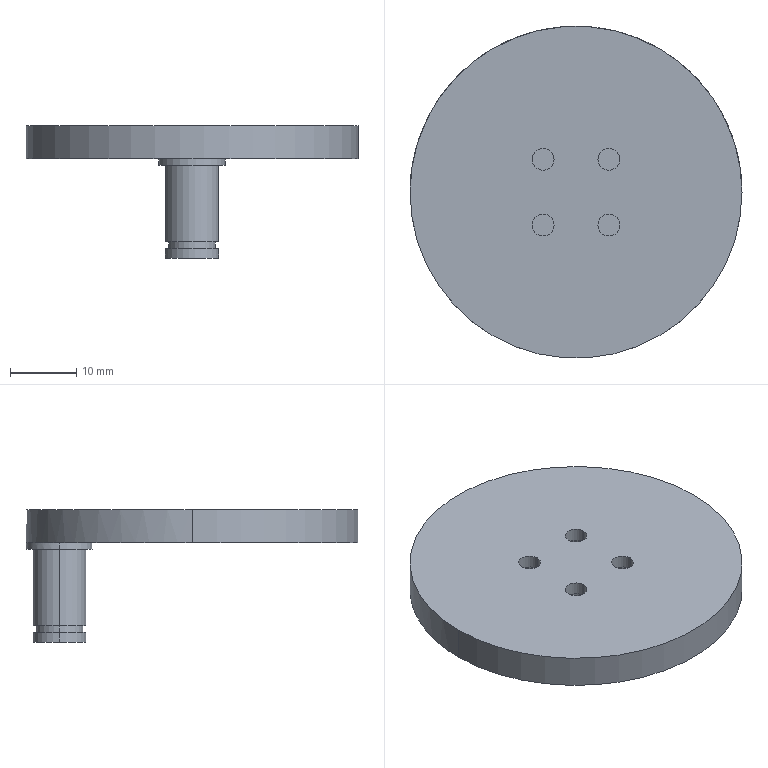Part | SolidWorks | features MirrorStock 1 | 1 solid | 36 faces | box 50 x 50 x 20 mm | volume 10180 mm3 | cylinder 26 | plane 10 | commonest cylinder face diameters 3.3 x8 6 x8 8 x4 7 x2 10 x2 50 x2
STEP:
#1=CARTESIAN_POINT('',(-4.,20.,-20.));
#2=VERTEX_POINT('',#1);
#3=CARTESIAN_POINT('',(4.,20.,-20.));
#4=VERTEX_POINT('',#3);
#5=CARTESIAN_POINT('',(0.,20.,-20.));
#6=DIRECTION('',(0.,0.,1.));
#7=DIRECTION('',(1.,0.,0.));
#8=AXIS2_PLACEMENT_3D('',#5,#6,#7);
#9=CIRCLE('',#8,4.);
#10=EDGE_CURVE('',#2,#4,#9,.T.);
#11=ORIENTED_EDGE('',*,*,#10,.T.);
#12=CARTESIAN_POINT('',(4.,20.,-18.5));
#13=VERTEX_POINT('',#12);
#14=CARTESIAN_POINT('',(4.,20.,-20.));
#15=DIRECTION('',(0.,0.,1.));
#16=VECTOR('',#15,1000.);
#17=LINE('',#14,#16);
#18=EDGE_CURVE('',#4,#13,#17,.T.);
#19=ORIENTED_EDGE('',*,*,#18,.T.);
#20=CARTESIAN_POINT('',(-4.,20.,-18.5));
#21=VERTEX_POINT('',#20);
#22=CARTESIAN_POINT('',(0.,20.,-18.5));
#23=DIRECTION('',(0.,0.,1.));
#24=DIRECTION('',(1.,0.,0.));
#25=AXIS2_PLACEMENT_3D('',#22,#23,#24);
#26=CIRCLE('',#25,4.);
#27=EDGE_CURVE('',#21,#13,#26,.T.);
#28=ORIENTED_EDGE('',*,*,#27,.F.);
#29=CARTESIAN_POINT('',(-4.,20.,-20.));
#30=DIRECTION('',(0.,0.,1.));
#31=VECTOR('',#30,1000.);
#32=LINE('',#29,#31);
#33=EDGE_CURVE('',#2,#21,#32,.T.);
#34=ORIENTED_EDGE('',*,*,#33,.F.);
#35=EDGE_LOOP('',(#11,#19,#28,#34));
#36=FACE_OUTER_BOUND('',#35,.T.);
#37=CARTESIAN_POINT('',(0.,20.,-20.));
#38=DIRECTION('',(0.,0.,1.));
#39=DIRECTION('',(-1.,0.,0.));
#40=AXIS2_PLACEMENT_3D('',#37,#38,#39);
#41=CYLINDRICAL_SURFACE('',#40,4.);
#42=ADVANCED_FACE('',(#36),#41,.T.);
#43=CARTESIAN_POINT('',(-3.5,20.,-17.5));
#44=VERTEX_POINT('',#43);
#45=CARTESIAN_POINT('',(3.5,20.,-17.5));
#46=VERTEX_POINT('',#45);
#47=CARTESIAN_POINT('',(0.,20.,-17.5));
#48=DIRECTION('',(0.,0.,1.));
#49=DIRECTION('',(1.,0.,0.));
#50=AXIS2_PLACEMENT_3D('',#47,#48,#49);
#51=CIRCLE('',#50,3.5);
#52=EDGE_CURVE('',#44,#46,#51,.T.);
#53=ORIENTED_EDGE('',*,*,#52,.F.);
#54=CARTESIAN_POINT('',(-3.5,20.,-18.5));
#55=VERTEX_POINT('',#54);
#56=CARTESIAN_POINT('',(-3.5,20.,-17.5));
#57=DIRECTION('',(0.,0.,-1.));
#58=VECTOR('',#57,1000.);
#59=LINE('',#56,#58);
#60=EDGE_CURVE('',#44,#55,#59,.T.);
#61=ORIENTED_EDGE('',*,*,#60,.T.);
#62=CARTESIAN_POINT('',(3.5,20.,-18.5));
#63=VERTEX_POINT('',#62);
#64=CARTESIAN_POINT('',(0.,20.,-18.5));
#65=DIRECTION('',(0.,0.,1.));
#66=DIRECTION('',(1.,0.,0.));
#67=AXIS2_PLACEMENT_3D('',#64,#65,#66);
#68=CIRCLE('',#67,3.5);
#69=EDGE_CURVE('',#55,#63,#68,.T.);
#70=ORIENTED_EDGE('',*,*,#69,.T.);
#71=CARTESIAN_POINT('',(3.5,20.,-17.5));
#72=DIRECTION('',(0.,0.,-1.));
#73=VECTOR('',#72,1000.);
#74=LINE('',#71,#73);
#75=EDGE_CURVE('',#46,#63,#74,.T.);
#76=ORIENTED_EDGE('',*,*,#75,.F.);
#77=EDGE_LOOP('',(#53,#61,#70,#76));
#78=FACE_OUTER_BOUND('',#77,.T.);
#79=CARTESIAN_POINT('',(0.,20.,-17.5));
#80=DIRECTION('',(0.,0.,-1.));
#81=DIRECTION('',(1.,0.,0.));
#82=AXIS2_PLACEMENT_3D('',#79,#80,#81);
#83=CYLINDRICAL_SURFACE('',#82,3.5);
#84=ADVANCED_FACE('',(#78),#83,.T.);
#85=CARTESIAN_POINT('',(-5.,20.,-6.));
#86=VERTEX_POINT('',#85);
#87=CARTESIAN_POINT('',(5.,20.,-6.));
#88=VERTEX_POINT('',#87);
#89=CARTESIAN_POINT('',(0.,20.,-6.));
#90=DIRECTION('',(0.,0.,1.));
#91=DIRECTION('',(1.,0.,0.));
#92=AXIS2_PLACEMENT_3D('',#89,#90,#91);
#93=CIRCLE('',#92,5.);
#94=EDGE_CURVE('',#86,#88,#93,.T.);
#95=ORIENTED_EDGE('',*,*,#94,.T.);
#96=CARTESIAN_POINT('',(5.,20.,-5.));
#97=VERTEX_POINT('',#96);
#98=CARTESIAN_POINT('',(5.,20.,-6.));
#99=DIRECTION('',(0.,0.,1.));
#100=VECTOR('',#99,1000.);
#101=LINE('',#98,#100);
#102=EDGE_CURVE('',#88,#97,#101,.T.);
#103=ORIENTED_EDGE('',*,*,#102,.T.);
#104=CARTESIAN_POINT('',(-5.,20.,-5.));
#105=VERTEX_POINT('',#104);
#106=CARTESIAN_POINT('',(0.,20.,-5.));
#107=DIRECTION('',(0.,0.,1.));
#108=DIRECTION('',(1.,0.,0.));
#109=AXIS2_PLACEMENT_3D('',#106,#107,#108);
#110=CIRCLE('',#109,5.);
#111=EDGE_CURVE('',#105,#97,#110,.T.);
#112=ORIENTED_EDGE('',*,*,#111,.F.);
#113=CARTESIAN_POINT('',(-5.,20.,-6.));
#114=DIRECTION('',(0.,0.,1.));
#115=VECTOR('',#114,1000.);
#116=LINE('',#113,#115);
#117=EDGE_CURVE('',#86,#105,#116,.T.);
#118=ORIENTED_EDGE('',*,*,#117,.F.);
#119=EDGE_LOOP('',(#95,#103,#112,#118));
#120=FACE_OUTER_BOUND('',#119,.T.);
#121=CARTESIAN_POINT('',(0.,20.,-6.));
#122=DIRECTION('',(0.,0.,1.));
#123=DIRECTION('',(-1.,0.,0.));
#124=AXIS2_PLACEMENT_3D('',#121,#122,#123);
#125=CYLINDRICAL_SURFACE('',#124,5.);
#126=ADVANCED_FACE('',(#120),#125,.T.);
#127=CARTESIAN_POINT('',(-7.95,4.95,-2.));
#128=VERTEX_POINT('',#127);
#129=CARTESIAN_POINT('',(-1.95,4.95,-2.));
#130=VERTEX_POINT('',#129);
#131=CARTESIAN_POINT('',(-4.95,4.95,-2.));
#132=DIRECTION('',(0.,0.,-1.));
#133=DIRECTION('',(-1.,0.,0.));
#134=AXIS2_PLACEMENT_3D('',#131,#132,#133);
#135=CIRCLE('',#134,3.);
#136=EDGE_CURVE('',#128,#130,#135,.T.);
#137=ORIENTED_EDGE('',*,*,#136,.F.);
#138=CARTESIAN_POINT('',(-7.95,4.95,-5.));
#139=VERTEX_POINT('',#138);
#140=CARTESIAN_POINT('',(-7.95,4.95,-2.));
#141=DIRECTION('',(0.,0.,-1.));
#142=VECTOR('',#141,1000.);
#143=LINE('',#140,#142);
#144=EDGE_CURVE('',#128,#139,#143,.T.);
#145=ORIENTED_EDGE('',*,*,#144,.T.);
#146=CARTESIAN_POINT('',(-1.95,4.95,-5.));
#147=VERTEX_POINT('',#146);
#148=CARTESIAN_POINT('',(-4.95,4.95,-5.));
#149=DIRECTION('',(0.,0.,-1.));
#150=DIRECTION('',(-1.,0.,0.));
#151=AXIS2_PLACEMENT_3D('',#148,#149,#150);
#152=CIRCLE('',#151,3.);
#153=EDGE_CURVE('',#139,#147,#152,.T.);
#154=ORIENTED_EDGE('',*,*,#153,.T.);
#155=CARTESIAN_POINT('',(-1.95,4.95,-2.));
#156=DIRECTION('',(0.,0.,-1.));
#157=VECTOR('',#156,1000.);
#158=LINE('',#155,#157);
#159=EDGE_CURVE('',#130,#147,#158,.T.);
#160=ORIENTED_EDGE('',*,*,#159,.F.);
#161=EDGE_LOOP('',(#137,#145,#154,#160));
#162=FACE_OUTER_BOUND('',#161,.T.);
#163=CARTESIAN_POINT('',(-4.95,4.95,-2.));
#164=DIRECTION('',(0.,0.,-1.));
#165=DIRECTION('',(1.,0.,0.));
#166=AXIS2_PLACEMENT_3D('',#163,#164,#165);
#167=CYLINDRICAL_SURFACE('',#166,3.);
#168=ADVANCED_FACE('',(#162),#167,.F.);
#169=CARTESIAN_POINT('',(1.95,4.95,-2.));
#170=VERTEX_POINT('',#169);
#171=CARTESIAN_POINT('',(7.95,4.95,-2.));
#172=VERTEX_POINT('',#171);
#173=CARTESIAN_POINT('',(4.95,4.95,-2.));
#174=DIRECTION('',(0.,0.,-1.));
#175=DIRECTION('',(-1.,0.,0.));
#176=AXIS2_PLACEMENT_3D('',#173,#174,#175);
#177=CIRCLE('',#176,3.);
#178=EDGE_CURVE('',#170,#172,#177,.T.);
#179=ORIENTED_EDGE('',*,*,#178,.F.);
#180=CARTESIAN_POINT('',(1.95,4.95,-5.));
#181=VERTEX_POINT('',#180);
#182=CARTESIAN_POINT('',(1.95,4.95,-2.));
#183=DIRECTION('',(0.,0.,-1.));
#184=VECTOR('',#183,1000.);
#185=LINE('',#182,#184);
#186=EDGE_CURVE('',#170,#181,#185,.T.);
#187=ORIENTED_EDGE('',*,*,#186,.T.);
#188=CARTESIAN_POINT('',(7.95,4.95,-5.));
#189=VERTEX_POINT('',#188);
#190=CARTESIAN_POINT('',(4.95,4.95,-5.));
#191=DIRECTION('',(0.,0.,-1.));
#192=DIRECTION('',(-1.,0.,0.));
#193=AXIS2_PLACEMENT_3D('',#190,#191,#192);
#194=CIRCLE('',#193,3.);
#195=EDGE_CURVE('',#181,#189,#194,.T.);
#196=ORIENTED_EDGE('',*,*,#195,.T.);
#197=CARTESIAN_POINT('',(7.95,4.95,-2.));
#198=DIRECTION('',(0.,0.,-1.));
#199=VECTOR('',#198,1000.);
#200=LINE('',#197,#199);
#201=EDGE_CURVE('',#172,#189,#200,.T.);
#202=ORIENTED_EDGE('',*,*,#201,.F.);
#203=EDGE_LOOP('',(#179,#187,#196,#202));
#204=FACE_OUTER_BOUND('',#203,.T.);
#205=CARTESIAN_POINT('',(4.95,4.95,-2.));
#206=DIRECTION('',(0.,0.,-1.));
#207=DIRECTION('',(1.,0.,0.));
#208=AXIS2_PLACEMENT_3D('',#205,#206,#207);
#209=CYLINDRICAL_SURFACE('',#208,3.);
#210=ADVANCED_FACE('',(#204),#209,.F.);
#211=CARTESIAN_POINT('',(1.95,-4.95,-2.));
#212=VERTEX_POINT('',#211);
#213=CARTESIAN_POINT('',(7.95,-4.95,-2.));
#214=VERTEX_POINT('',#213);
#215=CARTESIAN_POINT('',(4.95,-4.95,-2.));
#216=DIRECTION('',(0.,0.,-1.));
#217=DIRECTION('',(-1.,0.,0.));
#218=AXIS2_PLACEMENT_3D('',#215,#216,#217);
#219=CIRCLE('',#218,3.);
#220=EDGE_CURVE('',#212,#214,#219,.T.);
#221=ORIENTED_EDGE('',*,*,#220,.F.);
#222=CARTESIAN_POINT('',(1.95,-4.95,-5.));
#223=VERTEX_POINT('',#222);
#224=CARTESIAN_POINT('',(1.95,-4.95,-2.));
#225=DIRECTION('',(0.,0.,-1.));
#226=VECTOR('',#225,1000.);
#227=LINE('',#224,#226);
#228=EDGE_CURVE('',#212,#223,#227,.T.);
#229=ORIENTED_EDGE('',*,*,#228,.T.);
#230=CARTESIAN_POINT('',(7.95,-4.95,-5.));
#231=VERTEX_POINT('',#230);
#232=CARTESIAN_POINT('',(4.95,-4.95,-5.));
#233=DIRECTION('',(0.,0.,-1.));
#234=DIRECTION('',(-1.,0.,0.));
#235=AXIS2_PLACEMENT_3D('',#232,#233,#234);
#236=CIRCLE('',#235,3.);
#237=EDGE_CURVE('',#223,#231,#236,.T.);
#238=ORIENTED_EDGE('',*,*,#237,.T.);
#239=CARTESIAN_POINT('',(7.95,-4.95,-2.));
#240=DIRECTION('',(0.,0.,-1.));
#241=VECTOR('',#240,1000.);
#242=LINE('',#239,#241);
#243=EDGE_CURVE('',#214,#231,#242,.T.);
#244=ORIENTED_EDGE('',*,*,#243,.F.);
#245=EDGE_LOOP('',(#221,#229,#238,#244));
#246=FACE_OUTER_BOUND('',#245,.T.);
#247=CARTESIAN_POINT('',(4.95,-4.95,-2.));
#248=DIRECTION('',(0.,0.,-1.));
#249=DIRECTION('',(1.,0.,0.));
#250=AXIS2_PLACEMENT_3D('',#247,#248,#249);
#251=CYLINDRICAL_SURFACE('',#250,3.);
#252=ADVANCED_FACE('',(#246),#251,.F.);
#253=CARTESIAN_POINT('',(-7.95,-4.95,-2.));
#254=VERTEX_POINT('',#253);
#255=CARTESIAN_POINT('',(-1.95,-4.95,-2.));
#256=VERTEX_POINT('',#255);
#257=CARTESIAN_POINT('',(-4.95,-4.95,-2.));
#258=DIRECTION('',(0.,0.,-1.));
#259=DIRECTION('',(-1.,0.,0.));
#260=AXIS2_PLACEMENT_3D('',#257,#258,#259);
#261=CIRCLE('',#260,3.);
#262=EDGE_CURVE('',#254,#256,#261,.T.);
#263=ORIENTED_EDGE('',*,*,#262,.F.);
#264=CARTESIAN_POINT('',(-7.95,-4.95,-5.));
#265=VERTEX_POINT('',#264);
#266=CARTESIAN_POINT('',(-7.95,-4.95,-2.));
#267=DIRECTION('',(0.,0.,-1.));
#268=VECTOR('',#267,1000.);
#269=LINE('',#266,#268);
#270=EDGE_CURVE('',#254,#265,#269,.T.);
#271=ORIENTED_EDGE('',*,*,#270,.T.);
#272=CARTESIAN_POINT('',(-1.95,-4.95,-5.));
#273=VERTEX_POINT('',#272);
#274=CARTESIAN_POINT('',(-4.95,-4.95,-5.));
#275=DIRECTION('',(0.,0.,-1.));
#276=DIRECTION('',(-1.,0.,0.));
#277=AXIS2_PLACEMENT_3D('',#274,#275,#276);
#278=CIRCLE('',#277,3.);
#279=EDGE_CURVE('',#265,#273,#278,.T.);
#280=ORIENTED_EDGE('',*,*,#279,.T.);
#281=CARTESIAN_POINT('',(-1.95,-4.95,-2.));
#282=DIRECTION('',(0.,0.,-1.));
#283=VECTOR('',#282,1000.);
#284=LINE('',#281,#283);
#285=EDGE_CURVE('',#256,#273,#284,.T.);
#286=ORIENTED_EDGE('',*,*,#285,.F.);
#287=EDGE_LOOP('',(#263,#271,#280,#286));
#288=FACE_OUTER_BOUND('',#287,.T.);
#289=CARTESIAN_POINT('',(-4.95,-4.95,-2.));
#290=DIRECTION('',(0.,0.,-1.));
#291=DIRECTION('',(1.,0.,0.));
#292=AXIS2_PLACEMENT_3D('',#289,#290,#291);
#293=CYLINDRICAL_SURFACE('',#292,3.);
#294=ADVANCED_FACE('',(#288),#293,.F.);
#295=CARTESIAN_POINT('',(-3.3,-4.95,-2.));
#296=VERTEX_POINT('',#295);
#297=CARTESIAN_POINT('',(-6.6,-4.95,-2.));
#298=VERTEX_POINT('',#297);
#299=CARTESIAN_POINT('',(-4.95,-4.95,-2.));
#300=DIRECTION('',(0.,0.,1.));
#301=DIRECTION('',(-1.,0.,0.));
#302=AXIS2_PLACEMENT_3D('',#299,#300,#301);
#303=CIRCLE('',#302,1.65);
#304=EDGE_CURVE('',#296,#298,#303,.T.);
#305=ORIENTED_EDGE('',*,*,#304,.F.);
#306=CARTESIAN_POINT('',(-3.3,-4.95,0.));
#307=VERTEX_POINT('',#306);
#308=CARTESIAN_POINT('',(-3.3,-4.95,-10.));
#309=DIRECTION('',(0.,0.,1.));
#310=VECTOR('',#309,1000.);
#311=LINE('',#308,#310);
#312=EDGE_CURVE('',#296,#307,#311,.T.);
#313=ORIENTED_EDGE('',*,*,#312,.T.);
#314=CARTESIAN_POINT('',(-6.6,-4.95,0.));
#315=VERTEX_POINT('',#314);
#316=CARTESIAN_POINT('',(-4.95,-4.95,0.));
#317=DIRECTION('',(0.,0.,-1.));
#318=DIRECTION('',(0.,-1.,0.));
#319=AXIS2_PLACEMENT_3D('',#316,#317,#318);
#320=CIRCLE('',#319,1.65);
#321=EDGE_CURVE('',#315,#307,#320,.T.);
#322=ORIENTED_EDGE('',*,*,#321,.F.);
#323=CARTESIAN_POINT('',(-6.6,-4.95,-10.));
#324=DIRECTION('',(0.,0.,1.));
#325=VECTOR('',#324,1000.);
#326=LINE('',#323,#325);
#327=EDGE_CURVE('',#298,#315,#326,.T.);
#328=ORIENTED_EDGE('',*,*,#327,.F.);
#329=EDGE_LOOP('',(#305,#313,#322,#328));
#330=FACE_OUTER_BOUND('',#329,.T.);
#331=CARTESIAN_POINT('',(-4.95,-4.95,-10.));
#332=DIRECTION('',(0.,0.,1.));
#333=DIRECTION('',(-1.,0.,0.));
#334=AXIS2_PLACEMENT_3D('',#331,#332,#333);
#335=CYLINDRICAL_SURFACE('',#334,1.65);
#336=ADVANCED_FACE('',(#330),#335,.F.);
#337=CARTESIAN_POINT('',(6.6,-4.95,-2.));
#338=VERTEX_POINT('',#337);
#339=CARTESIAN_POINT('',(3.3,-4.95,-2.));
#340=VERTEX_POINT('',#339);
#341=CARTESIAN_POINT('',(4.95,-4.95,-2.));
#342=DIRECTION('',(0.,0.,1.));
#343=DIRECTION('',(-1.,0.,0.));
#344=AXIS2_PLACEMENT_3D('',#341,#342,#343);
#345=CIRCLE('',#344,1.65);
#346=EDGE_CURVE('',#338,#340,#345,.T.);
#347=ORIENTED_EDGE('',*,*,#346,.F.);
#348=CARTESIAN_POINT('',(6.6,-4.95,0.));
#349=VERTEX_POINT('',#348);
#350=CARTESIAN_POINT('',(6.6,-4.95,-10.));
#351=DIRECTION('',(0.,0.,1.));
#352=VECTOR('',#351,1000.);
#353=LINE('',#350,#352);
#354=EDGE_CURVE('',#338,#349,#353,.T.);
#355=ORIENTED_EDGE('',*,*,#354,.T.);
#356=CARTESIAN_POINT('',(3.3,-4.95,0.));
#357=VERTEX_POINT('',#356);
#358=CARTESIAN_POINT('',(4.95,-4.95,0.));
#359=DIRECTION('',(0.,0.,-1.));
#360=DIRECTION('',(1.,0.,0.));
#361=AXIS2_PLACEMENT_3D('',#358,#359,#360);
#362=CIRCLE('',#361,1.65);
#363=EDGE_CURVE('',#357,#349,#362,.T.);
#364=ORIENTED_EDGE('',*,*,#363,.F.);
#365=CARTESIAN_POINT('',(3.3,-4.95,-10.));
#366=DIRECTION('',(0.,0.,1.));
#367=VECTOR('',#366,1000.);
#368=LINE('',#365,#367);
#369=EDGE_CURVE('',#340,#357,#368,.T.);
#370=ORIENTED_EDGE('',*,*,#369,.F.);
#371=EDGE_LOOP('',(#347,#355,#364,#370));
#372=FACE_OUTER_BOUND('',#371,.T.);
#373=CARTESIAN_POINT('',(4.95,-4.95,-10.));
#374=DIRECTION('',(0.,0.,1.));
#375=DIRECTION('',(-1.,0.,0.));
#376=AXIS2_PLACEMENT_3D('',#373,#374,#375);
#377=CYLINDRICAL_SURFACE('',#376,1.65);
#378=ADVANCED_FACE('',(#372),#377,.F.);
#379=CARTESIAN_POINT('',(6.6,4.95,-2.));
#380=VERTEX_POINT('',#379);
#381=CARTESIAN_POINT('',(3.3,4.95,-2.));
#382=VERTEX_POINT('',#381);
#383=CARTESIAN_POINT('',(4.95,4.95,-2.));
#384=DIRECTION('',(0.,0.,1.));
#385=DIRECTION('',(-1.,0.,0.));
#386=AXIS2_PLACEMENT_3D('',#383,#384,#385);
#387=CIRCLE('',#386,1.65);
#388=EDGE_CURVE('',#380,#382,#387,.T.);
#389=ORIENTED_EDGE('',*,*,#388,.F.);
#390=CARTESIAN_POINT('',(6.6,4.95,0.));
#391=VERTEX_POINT('',#390);
#392=CARTESIAN_POINT('',(6.6,4.95,-10.));
#393=DIRECTION('',(0.,0.,1.));
#394=VECTOR('',#393,1000.);
#395=LINE('',#392,#394);
#396=EDGE_CURVE('',#380,#391,#395,.T.);
#397=ORIENTED_EDGE('',*,*,#396,.T.);
#398=CARTESIAN_POINT('',(3.3,4.95,0.));
#399=VERTEX_POINT('',#398);
#400=CARTESIAN_POINT('',(4.95,4.95,0.));
#401=DIRECTION('',(0.,0.,-1.));
#402=DIRECTION('',(0.,1.,0.));
#403=AXIS2_PLACEMENT_3D('',#400,#401,#402);
#404=CIRCLE('',#403,1.65);
#405=EDGE_CURVE('',#399,#391,#404,.T.);
#406=ORIENTED_EDGE('',*,*,#405,.F.);
#407=CARTESIAN_POINT('',(3.3,4.95,-10.));
#408=DIRECTION('',(0.,0.,1.));
#409=VECTOR('',#408,1000.);
#410=LINE('',#407,#409);
#411=EDGE_CURVE('',#382,#399,#410,.T.);
#412=ORIENTED_EDGE('',*,*,#411,.F.);
#413=EDGE_LOOP('',(#389,#397,#406,#412));
#414=FACE_OUTER_BOUND('',#413,.T.);
#415=CARTESIAN_POINT('',(4.95,4.95,-10.));
#416=DIRECTION('',(0.,0.,1.));
#417=DIRECTION('',(-1.,0.,0.));
#418=AXIS2_PLACEMENT_3D('',#415,#416,#417);
#419=CYLINDRICAL_SURFACE('',#418,1.65);
#420=ADVANCED_FACE('',(#414),#419,.F.);
#421=CARTESIAN_POINT('',(-3.3,4.95,-2.));
#422=VERTEX_POINT('',#421);
#423=CARTESIAN_POINT('',(-6.6,4.95,-2.));
#424=VERTEX_POINT('',#423);
#425=CARTESIAN_POINT('',(-4.95,4.95,-2.));
#426=DIRECTION('',(0.,0.,1.));
#427=DIRECTION('',(-1.,0.,0.));
#428=AXIS2_PLACEMENT_3D('',#425,#426,#427);
#429=CIRCLE('',#428,1.65);
#430=EDGE_CURVE('',#422,#424,#429,.T.);
#431=ORIENTED_EDGE('',*,*,#430,.F.);
#432=CARTESIAN_POINT('',(-3.3,4.95,0.));
#433=VERTEX_POINT('',#432);
#434=CARTESIAN_POINT('',(-3.3,4.95,-10.));
#435=DIRECTION('',(0.,0.,1.));
#436=VECTOR('',#435,1000.);
#437=LINE('',#434,#436);
#438=EDGE_CURVE('',#422,#433,#437,.T.);
#439=ORIENTED_EDGE('',*,*,#438,.T.);
#440=CARTESIAN_POINT('',(-6.6,4.95,0.));
#441=VERTEX_POINT('',#440);
#442=CARTESIAN_POINT('',(-4.95,4.95,0.));
#443=DIRECTION('',(0.,0.,-1.));
#444=DIRECTION('',(-1.,0.,0.));
#445=AXIS2_PLACEMENT_3D('',#442,#443,#444);
#446=CIRCLE('',#445,1.65);
#447=EDGE_CURVE('',#441,#433,#446,.T.);
#448=ORIENTED_EDGE('',*,*,#447,.F.);
#449=CARTESIAN_POINT('',(-6.6,4.95,-10.));
#450=DIRECTION('',(0.,0.,1.));
#451=VECTOR('',#450,1000.);
#452=LINE('',#449,#451);
#453=EDGE_CURVE('',#424,#441,#452,.T.);
#454=ORIENTED_EDGE('',*,*,#453,.F.);
#455=EDGE_LOOP('',(#431,#439,#448,#454));
#456=FACE_OUTER_BOUND('',#455,.T.);
#457=CARTESIAN_POINT('',(-4.95,4.95,-10.));
#458=DIRECTION('',(0.,0.,1.));
#459=DIRECTION('',(-1.,0.,0.));
#460=AXIS2_PLACEMENT_3D('',#457,#458,#459);
#461=CYLINDRICAL_SURFACE('',#460,1.65);
#462=ADVANCED_FACE('',(#456),#461,.F.);
#463=CARTESIAN_POINT('',(-25.,0.,-5.));
#464=VERTEX_POINT('',#463);
#465=CARTESIAN_POINT('',(25.,0.,-5.));
#466=VERTEX_POINT('',#465);
#467=CARTESIAN_POINT('',(0.,0.,-5.));
#468=DIRECTION('',(0.,0.,1.));
#469=DIRECTION('',(1.,0.,0.));
#470=AXIS2_PLACEMENT_3D('',#467,#468,#469);
#471=CIRCLE('',#470,25.);
#472=EDGE_CURVE('',#464,#466,#471,.T.);
#473=ORIENTED_EDGE('',*,*,#472,.T.);
#474=CARTESIAN_POINT('',(25.,0.,0.));
#475=VERTEX_POINT('',#474);
#476=CARTESIAN_POINT('',(25.,0.,-5.));
#477=DIRECTION('',(0.,0.,1.));
#478=VECTOR('',#477,1000.);
#479=LINE('',#476,#478);
#480=EDGE_CURVE('',#466,#475,#479,.T.);
#481=ORIENTED_EDGE('',*,*,#480,.T.);
#482=CARTESIAN_POINT('',(-25.,0.,0.));
#483=VERTEX_POINT('',#482);
#484=CARTESIAN_POINT('',(0.,0.,0.));
#485=DIRECTION('',(0.,0.,1.));
#486=DIRECTION('',(1.,0.,0.));
#487=AXIS2_PLACEMENT_3D('',#484,#485,#486);
#488=CIRCLE('',#487,25.);
#489=EDGE_CURVE('',#483,#475,#488,.T.);
#490=ORIENTED_EDGE('',*,*,#489,.F.);
#491=CARTESIAN_POINT('',(-25.,0.,-5.));
#492=DIRECTION('',(0.,0.,1.));
#493=VECTOR('',#492,1000.);
#494=LINE('',#491,#493);
#495=EDGE_CURVE('',#464,#483,#494,.T.);
#496=ORIENTED_EDGE('',*,*,#495,.F.);
#497=EDGE_LOOP('',(#473,#481,#490,#496));
#498=FACE_OUTER_BOUND('',#497,.T.);
#499=CARTESIAN_POINT('',(0.,0.,-5.));
#500=DIRECTION('',(0.,0.,1.));
#501=DIRECTION('',(-1.,0.,0.));
#502=AXIS2_PLACEMENT_3D('',#499,#500,#501);
#503=CYLINDRICAL_SURFACE('',#502,25.);
#504=ADVANCED_FACE('',(#498),#503,.T.);
#505=CARTESIAN_POINT('',(-4.,20.,-17.5));
#506=VERTEX_POINT('',#505);
#507=CARTESIAN_POINT('',(4.,20.,-17.5));
#508=VERTEX_POINT('',#507);
#509=CARTESIAN_POINT('',(0.,20.,-17.5));
#510=DIRECTION('',(0.,0.,1.));
#511=DIRECTION('',(1.,0.,0.));
#512=AXIS2_PLACEMENT_3D('',#509,#510,#511);
#513=CIRCLE('',#512,4.);
#514=EDGE_CURVE('',#506,#508,#513,.T.);
#515=ORIENTED_EDGE('',*,*,#514,.T.);
#516=CARTESIAN_POINT('',(4.,20.,-6.));
#517=VERTEX_POINT('',#516);
#518=CARTESIAN_POINT('',(4.,20.,-20.));
#519=DIRECTION('',(0.,0.,1.));
#520=VECTOR('',#519,1000.);
#521=LINE('',#518,#520);
#522=EDGE_CURVE('',#508,#517,#521,.T.);
#523=ORIENTED_EDGE('',*,*,#522,.T.);
#524=CARTESIAN_POINT('',(-4.,20.,-6.));
#525=VERTEX_POINT('',#524);
#526=CARTESIAN_POINT('',(0.,20.,-6.));
#527=DIRECTION('',(0.,0.,1.));
#528=DIRECTION('',(1.,0.,0.));
#529=AXIS2_PLACEMENT_3D('',#526,#527,#528);
#530=CIRCLE('',#529,4.);
#531=EDGE_CURVE('',#525,#517,#530,.T.);
#532=ORIENTED_EDGE('',*,*,#531,.F.);
#533=CARTESIAN_POINT('',(-4.,20.,-20.));
#534=DIRECTION('',(0.,0.,1.));
#535=VECTOR('',#534,1000.);
#536=LINE('',#533,#535);
#537=EDGE_CURVE('',#506,#525,#536,.T.);
#538=ORIENTED_EDGE('',*,*,#537,.F.);
#539=EDGE_LOOP('',(#515,#523,#532,#538));
#540=FACE_OUTER_BOUND('',#539,.T.);
#541=CARTESIAN_POINT('',(0.,20.,-20.));
#542=DIRECTION('',(0.,0.,1.));
#543=DIRECTION('',(-1.,0.,0.));
#544=AXIS2_PLACEMENT_3D('',#541,#542,#543);
#545=CYLINDRICAL_SURFACE('',#544,4.);
#546=ADVANCED_FACE('',(#540),#545,.T.);
#547=ORIENTED_EDGE('',*,*,#522,.F.);
#548=CARTESIAN_POINT('',(0.,20.,-17.5));
#549=DIRECTION('',(0.,0.,1.));
#550=DIRECTION('',(1.,0.,0.));
#551=AXIS2_PLACEMENT_3D('',#548,#549,#550);
#552=CIRCLE('',#551,4.);
#553=EDGE_CURVE('',#508,#506,#552,.T.);
#554=ORIENTED_EDGE('',*,*,#553,.T.);
#555=ORIENTED_EDGE('',*,*,#537,.T.);
#556=CARTESIAN_POINT('',(0.,20.,-6.));
#557=DIRECTION('',(0.,0.,1.));
#558=DIRECTION('',(1.,0.,0.));
#559=AXIS2_PLACEMENT_3D('',#556,#557,#558);
#560=CIRCLE('',#559,4.);
#561=EDGE_CURVE('',#517,#525,#560,.T.);
#562=ORIENTED_EDGE('',*,*,#561,.F.);
#563=EDGE_LOOP('',(#547,#554,#555,#562));
#564=FACE_OUTER_BOUND('',#563,.T.);
#565=CARTESIAN_POINT('',(0.,20.,-20.));
#566=DIRECTION('',(0.,0.,1.));
#567=DIRECTION('',(-1.,0.,0.));
#568=AXIS2_PLACEMENT_3D('',#565,#566,#567);
#569=CYLINDRICAL_SURFACE('',#568,4.);
#570=ADVANCED_FACE('',(#564),#569,.T.);
#571=CARTESIAN_POINT('',(4.95,4.95,-5.));
#572=DIRECTION('',(0.,0.,-1.));
#573=DIRECTION('',(-1.,0.,0.));
#574=AXIS2_PLACEMENT_3D('',#571,#572,#573);
#575=CIRCLE('',#574,3.);
#576=EDGE_CURVE('',#189,#181,#575,.T.);
#577=ORIENTED_EDGE('',*,*,#576,.F.);
#578=ORIENTED_EDGE('',*,*,#195,.F.);
#579=EDGE_LOOP('',(#577,#578));
#580=FACE_BOUND('',#579,.T.);
#581=CARTESIAN_POINT('',(-4.95,4.95,-5.));
#582=DIRECTION('',(0.,0.,-1.));
#583=DIRECTION('',(-1.,0.,0.));
#584=AXIS2_PLACEMENT_3D('',#581,#582,#583);
#585=CIRCLE('',#584,3.);
#586=EDGE_CURVE('',#147,#139,#585,.T.);
#587=ORIENTED_EDGE('',*,*,#586,.F.);
#588=ORIENTED_EDGE('',*,*,#153,.F.);
#589=EDGE_LOOP('',(#587,#588));
#590=FACE_BOUND('',#589,.T.);
#591=CARTESIAN_POINT('',(-4.95,-4.95,-5.));
#592=DIRECTION('',(0.,0.,-1.));
#593=DIRECTION('',(-1.,0.,0.));
#594=AXIS2_PLACEMENT_3D('',#591,#592,#593);
#595=CIRCLE('',#594,3.);
#596=EDGE_CURVE('',#273,#265,#595,.T.);
#597=ORIENTED_EDGE('',*,*,#596,.F.);
#598=ORIENTED_EDGE('',*,*,#279,.F.);
#599=EDGE_LOOP('',(#597,#598));
#600=FACE_BOUND('',#599,.T.);
#601=CARTESIAN_POINT('',(4.95,-4.95,-5.));
#602=DIRECTION('',(0.,0.,-1.));
#603=DIRECTION('',(-1.,0.,0.));
#604=AXIS2_PLACEMENT_3D('',#601,#602,#603);
#605=CIRCLE('',#604,3.);
#606=EDGE_CURVE('',#231,#223,#605,.T.);
#607=ORIENTED_EDGE('',*,*,#606,.F.);
#608=ORIENTED_EDGE('',*,*,#237,.F.);
#609=EDGE_LOOP('',(#607,#608));
#610=FACE_BOUND('',#609,.T.);
#611=CARTESIAN_POINT('',(0.,25.,-5.));
#612=VERTEX_POINT('',#611);
#613=CARTESIAN_POINT('',(0.,0.,-5.));
#614=DIRECTION('',(0.,0.,1.));
#615=DIRECTION('',(1.,0.,0.));
#616=AXIS2_PLACEMENT_3D('',#613,#614,#615);
#617=CIRCLE('',#616,25.);
#618=EDGE_CURVE('',#612,#464,#617,.T.);
#619=ORIENTED_EDGE('',*,*,#618,.F.);
#620=CARTESIAN_POINT('',(0.,20.,-5.));
#621=DIRECTION('',(0.,0.,1.));
#622=DIRECTION('',(1.,0.,0.));
#623=AXIS2_PLACEMENT_3D('',#620,#621,#622);
#624=CIRCLE('',#623,5.);
#625=EDGE_CURVE('',#612,#105,#624,.T.);
#626=ORIENTED_EDGE('',*,*,#625,.T.);
#627=ORIENTED_EDGE('',*,*,#111,.T.);
#628=CARTESIAN_POINT('',(0.,20.,-5.));
#629=DIRECTION('',(0.,0.,1.));
#630=DIRECTION('',(1.,0.,0.));
#631=AXIS2_PLACEMENT_3D('',#628,#629,#630);
#632=CIRCLE('',#631,5.);
#633=EDGE_CURVE('',#97,#612,#632,.T.);
#634=ORIENTED_EDGE('',*,*,#633,.T.);
#635=CARTESIAN_POINT('',(0.,0.,-5.));
#636=DIRECTION('',(0.,0.,1.));
#637=DIRECTION('',(1.,0.,0.));
#638=AXIS2_PLACEMENT_3D('',#635,#636,#637);
#639=CIRCLE('',#638,25.);
#640=EDGE_CURVE('',#466,#612,#639,.T.);
#641=ORIENTED_EDGE('',*,*,#640,.F.);
#642=ORIENTED_EDGE('',*,*,#472,.F.);
#643=EDGE_LOOP('',(#619,#626,#627,#634,#641,#642));
#644=FACE_OUTER_BOUND('',#643,.T.);
#645=CARTESIAN_POINT('',(0.,0.,-5.));
#646=DIRECTION('',(0.,0.,-1.));
#647=DIRECTION('',(1.,0.,0.));
#648=AXIS2_PLACEMENT_3D('',#645,#646,#647);
#649=PLANE('',#648);
#650=ADVANCED_FACE('',(#580,#590,#600,#610,#644),#649,.T.);
#651=ORIENTED_EDGE('',*,*,#480,.F.);
#652=ORIENTED_EDGE('',*,*,#640,.T.);
#653=ORIENTED_EDGE('',*,*,#618,.T.);
#654=ORIENTED_EDGE('',*,*,#495,.T.);
#655=CARTESIAN_POINT('',(0.,0.,0.));
#656=DIRECTION('',(0.,0.,1.));
#657=DIRECTION('',(1.,0.,0.));
#658=AXIS2_PLACEMENT_3D('',#655,#656,#657);
#659=CIRCLE('',#658,25.);
#660=EDGE_CURVE('',#475,#483,#659,.T.);
#661=ORIENTED_EDGE('',*,*,#660,.F.);
#662=EDGE_LOOP('',(#651,#652,#653,#654,#661));
#663=FACE_OUTER_BOUND('',#662,.T.);
#664=CARTESIAN_POINT('',(0.,0.,-5.));
#665=DIRECTION('',(0.,0.,1.));
#666=DIRECTION('',(-1.,0.,0.));
#667=AXIS2_PLACEMENT_3D('',#664,#665,#666);
#668=CYLINDRICAL_SURFACE('',#667,25.);
#669=ADVANCED_FACE('',(#663),#668,.T.);
#670=ORIENTED_EDGE('',*,*,#321,.T.);
#671=CARTESIAN_POINT('',(-4.95,-4.95,0.));
#672=DIRECTION('',(0.,0.,-1.));
#673=DIRECTION('',(0.,-1.,0.));
#674=AXIS2_PLACEMENT_3D('',#671,#672,#673);
#675=CIRCLE('',#674,1.65);
#676=EDGE_CURVE('',#307,#315,#675,.T.);
#677=ORIENTED_EDGE('',*,*,#676,.T.);
#678=EDGE_LOOP('',(#670,#677));
#679=FACE_BOUND('',#678,.T.);
#680=ORIENTED_EDGE('',*,*,#363,.T.);
#681=CARTESIAN_POINT('',(4.95,-4.95,0.));
#682=DIRECTION('',(0.,0.,-1.));
#683=DIRECTION('',(1.,0.,0.));
#684=AXIS2_PLACEMENT_3D('',#681,#682,#683);
#685=CIRCLE('',#684,1.65);
#686=EDGE_CURVE('',#349,#357,#685,.T.);
#687=ORIENTED_EDGE('',*,*,#686,.T.);
#688=EDGE_LOOP('',(#680,#687));
#689=FACE_BOUND('',#688,.T.);
#690=ORIENTED_EDGE('',*,*,#405,.T.);
#691=CARTESIAN_POINT('',(4.95,4.95,0.));
#692=DIRECTION('',(0.,0.,-1.));
#693=DIRECTION('',(0.,1.,0.));
#694=AXIS2_PLACEMENT_3D('',#691,#692,#693);
#695=CIRCLE('',#694,1.65);
#696=EDGE_CURVE('',#391,#399,#695,.T.);
#697=ORIENTED_EDGE('',*,*,#696,.T.);
#698=EDGE_LOOP('',(#690,#697));
#699=FACE_BOUND('',#698,.T.);
#700=ORIENTED_EDGE('',*,*,#447,.T.);
#701=CARTESIAN_POINT('',(-4.95,4.95,0.));
#702=DIRECTION('',(0.,0.,-1.));
#703=DIRECTION('',(-1.,0.,0.));
#704=AXIS2_PLACEMENT_3D('',#701,#702,#703);
#705=CIRCLE('',#704,1.65);
#706=EDGE_CURVE('',#433,#441,#705,.T.);
#707=ORIENTED_EDGE('',*,*,#706,.T.);
#708=EDGE_LOOP('',(#700,#707));
#709=FACE_BOUND('',#708,.T.);
#710=ORIENTED_EDGE('',*,*,#489,.T.);
#711=ORIENTED_EDGE('',*,*,#660,.T.);
#712=EDGE_LOOP('',(#710,#711));
#713=FACE_OUTER_BOUND('',#712,.T.);
#714=CARTESIAN_POINT('',(0.,0.,0.));
#715=DIRECTION('',(0.,0.,-1.));
#716=DIRECTION('',(1.,0.,0.));
#717=AXIS2_PLACEMENT_3D('',#714,#715,#716);
#718=PLANE('',#717);
#719=ADVANCED_FACE('',(#679,#689,#699,#709,#713),#718,.F.);
#720=ORIENTED_EDGE('',*,*,#438,.F.);
#721=CARTESIAN_POINT('',(-4.95,4.95,-2.));
#722=DIRECTION('',(0.,0.,1.));
#723=DIRECTION('',(-1.,0.,0.));
#724=AXIS2_PLACEMENT_3D('',#721,#722,#723);
#725=CIRCLE('',#724,1.65);
#726=EDGE_CURVE('',#424,#422,#725,.T.);
#727=ORIENTED_EDGE('',*,*,#726,.F.);
#728=ORIENTED_EDGE('',*,*,#453,.T.);
#729=ORIENTED_EDGE('',*,*,#706,.F.);
#730=EDGE_LOOP('',(#720,#727,#728,#729));
#731=FACE_OUTER_BOUND('',#730,.T.);
#732=CARTESIAN_POINT('',(-4.95,4.95,-10.));
#733=DIRECTION('',(0.,0.,1.));
#734=DIRECTION('',(-1.,0.,0.));
#735=AXIS2_PLACEMENT_3D('',#732,#733,#734);
#736=CYLINDRICAL_SURFACE('',#735,1.65);
#737=ADVANCED_FACE('',(#731),#736,.F.);
#738=ORIENTED_EDGE('',*,*,#396,.F.);
#739=CARTESIAN_POINT('',(4.95,4.95,-2.));
#740=DIRECTION('',(0.,0.,1.));
#741=DIRECTION('',(-1.,0.,0.));
#742=AXIS2_PLACEMENT_3D('',#739,#740,#741);
#743=CIRCLE('',#742,1.65);
#744=EDGE_CURVE('',#382,#380,#743,.T.);
#745=ORIENTED_EDGE('',*,*,#744,.F.);
#746=ORIENTED_EDGE('',*,*,#411,.T.);
#747=ORIENTED_EDGE('',*,*,#696,.F.);
#748=EDGE_LOOP('',(#738,#745,#746,#747));
#749=FACE_OUTER_BOUND('',#748,.T.);
#750=CARTESIAN_POINT('',(4.95,4.95,-10.));
#751=DIRECTION('',(0.,0.,1.));
#752=DIRECTION('',(-1.,0.,0.));
#753=AXIS2_PLACEMENT_3D('',#750,#751,#752);
#754=CYLINDRICAL_SURFACE('',#753,1.65);
#755=ADVANCED_FACE('',(#749),#754,.F.);
#756=ORIENTED_EDGE('',*,*,#354,.F.);
#757=CARTESIAN_POINT('',(4.95,-4.95,-2.));
#758=DIRECTION('',(0.,0.,1.));
#759=DIRECTION('',(-1.,0.,0.));
#760=AXIS2_PLACEMENT_3D('',#757,#758,#759);
#761=CIRCLE('',#760,1.65);
#762=EDGE_CURVE('',#340,#338,#761,.T.);
#763=ORIENTED_EDGE('',*,*,#762,.F.);
#764=ORIENTED_EDGE('',*,*,#369,.T.);
#765=ORIENTED_EDGE('',*,*,#686,.F.);
#766=EDGE_LOOP('',(#756,#763,#764,#765));
#767=FACE_OUTER_BOUND('',#766,.T.);
#768=CARTESIAN_POINT('',(4.95,-4.95,-10.));
#769=DIRECTION('',(0.,0.,1.));
#770=DIRECTION('',(-1.,0.,0.));
#771=AXIS2_PLACEMENT_3D('',#768,#769,#770);
#772=CYLINDRICAL_SURFACE('',#771,1.65);
#773=ADVANCED_FACE('',(#767),#772,.F.);
#774=ORIENTED_EDGE('',*,*,#312,.F.);
#775=CARTESIAN_POINT('',(-4.95,-4.95,-2.));
#776=DIRECTION('',(0.,0.,1.));
#777=DIRECTION('',(-1.,0.,0.));
#778=AXIS2_PLACEMENT_3D('',#775,#776,#777);
#779=CIRCLE('',#778,1.65);
#780=EDGE_CURVE('',#298,#296,#779,.T.);
#781=ORIENTED_EDGE('',*,*,#780,.F.);
#782=ORIENTED_EDGE('',*,*,#327,.T.);
#783=ORIENTED_EDGE('',*,*,#676,.F.);
#784=EDGE_LOOP('',(#774,#781,#782,#783));
#785=FACE_OUTER_BOUND('',#784,.T.);
#786=CARTESIAN_POINT('',(-4.95,-4.95,-10.));
#787=DIRECTION('',(0.,0.,1.));
#788=DIRECTION('',(-1.,0.,0.));
#789=AXIS2_PLACEMENT_3D('',#786,#787,#788);
#790=CYLINDRICAL_SURFACE('',#789,1.65);
#791=ADVANCED_FACE('',(#785),#790,.F.);
#792=CARTESIAN_POINT('',(-4.95,-4.95,-2.));
#793=DIRECTION('',(0.,0.,-1.));
#794=DIRECTION('',(-1.,0.,0.));
#795=AXIS2_PLACEMENT_3D('',#792,#793,#794);
#796=CIRCLE('',#795,3.);
#797=EDGE_CURVE('',#256,#254,#796,.T.);
#798=ORIENTED_EDGE('',*,*,#797,.T.);
#799=ORIENTED_EDGE('',*,*,#262,.T.);
#800=EDGE_LOOP('',(#798,#799));
#801=FACE_OUTER_BOUND('',#800,.T.);
#802=ORIENTED_EDGE('',*,*,#780,.T.);
#803=ORIENTED_EDGE('',*,*,#304,.T.);
#804=EDGE_LOOP('',(#802,#803));
#805=FACE_BOUND('',#804,.T.);
#806=CARTESIAN_POINT('',(-4.95,-4.95,-2.));
#807=DIRECTION('',(0.,0.,1.));
#808=DIRECTION('',(-1.,0.,0.));
#809=AXIS2_PLACEMENT_3D('',#806,#807,#808);
#810=PLANE('',#809);
#811=ADVANCED_FACE('',(#801,#805),#810,.F.);
#812=ORIENTED_EDGE('',*,*,#270,.F.);
#813=ORIENTED_EDGE('',*,*,#797,.F.);
#814=ORIENTED_EDGE('',*,*,#285,.T.);
#815=ORIENTED_EDGE('',*,*,#596,.T.);
#816=EDGE_LOOP('',(#812,#813,#814,#815));
#817=FACE_OUTER_BOUND('',#816,.T.);
#818=CARTESIAN_POINT('',(-4.95,-4.95,-2.));
#819=DIRECTION('',(0.,0.,-1.));
#820=DIRECTION('',(1.,0.,0.));
#821=AXIS2_PLACEMENT_3D('',#818,#819,#820);
#822=CYLINDRICAL_SURFACE('',#821,3.);
#823=ADVANCED_FACE('',(#817),#822,.F.);
#824=CARTESIAN_POINT('',(4.95,-4.95,-2.));
#825=DIRECTION('',(0.,0.,-1.));
#826=DIRECTION('',(-1.,0.,0.));
#827=AXIS2_PLACEMENT_3D('',#824,#825,#826);
#828=CIRCLE('',#827,3.);
#829=EDGE_CURVE('',#214,#212,#828,.T.);
#830=ORIENTED_EDGE('',*,*,#829,.T.);
#831=ORIENTED_EDGE('',*,*,#220,.T.);
#832=EDGE_LOOP('',(#830,#831));
#833=FACE_OUTER_BOUND('',#832,.T.);
#834=ORIENTED_EDGE('',*,*,#762,.T.);
#835=ORIENTED_EDGE('',*,*,#346,.T.);
#836=EDGE_LOOP('',(#834,#835));
#837=FACE_BOUND('',#836,.T.);
#838=CARTESIAN_POINT('',(4.95,-4.95,-2.));
#839=DIRECTION('',(0.,0.,1.));
#840=DIRECTION('',(-1.,0.,0.));
#841=AXIS2_PLACEMENT_3D('',#838,#839,#840);
#842=PLANE('',#841);
#843=ADVANCED_FACE('',(#833,#837),#842,.F.);
#844=ORIENTED_EDGE('',*,*,#228,.F.);
#845=ORIENTED_EDGE('',*,*,#829,.F.);
#846=ORIENTED_EDGE('',*,*,#243,.T.);
#847=ORIENTED_EDGE('',*,*,#606,.T.);
#848=EDGE_LOOP('',(#844,#845,#846,#847));
#849=FACE_OUTER_BOUND('',#848,.T.);
#850=CARTESIAN_POINT('',(4.95,-4.95,-2.));
#851=DIRECTION('',(0.,0.,-1.));
#852=DIRECTION('',(1.,0.,0.));
#853=AXIS2_PLACEMENT_3D('',#850,#851,#852);
#854=CYLINDRICAL_SURFACE('',#853,3.);
#855=ADVANCED_FACE('',(#849),#854,.F.);
#856=CARTESIAN_POINT('',(4.95,4.95,-2.));
#857=DIRECTION('',(0.,0.,-1.));
#858=DIRECTION('',(-1.,0.,0.));
#859=AXIS2_PLACEMENT_3D('',#856,#857,#858);
#860=CIRCLE('',#859,3.);
#861=EDGE_CURVE('',#172,#170,#860,.T.);
#862=ORIENTED_EDGE('',*,*,#861,.T.);
#863=ORIENTED_EDGE('',*,*,#178,.T.);
#864=EDGE_LOOP('',(#862,#863));
#865=FACE_OUTER_BOUND('',#864,.T.);
#866=ORIENTED_EDGE('',*,*,#744,.T.);
#867=ORIENTED_EDGE('',*,*,#388,.T.);
#868=EDGE_LOOP('',(#866,#867));
#869=FACE_BOUND('',#868,.T.);
#870=CARTESIAN_POINT('',(4.95,4.95,-2.));
#871=DIRECTION('',(0.,0.,1.));
#872=DIRECTION('',(-1.,0.,0.));
#873=AXIS2_PLACEMENT_3D('',#870,#871,#872);
#874=PLANE('',#873);
#875=ADVANCED_FACE('',(#865,#869),#874,.F.);
#876=ORIENTED_EDGE('',*,*,#186,.F.);
#877=ORIENTED_EDGE('',*,*,#861,.F.);
#878=ORIENTED_EDGE('',*,*,#201,.T.);
#879=ORIENTED_EDGE('',*,*,#576,.T.);
#880=EDGE_LOOP('',(#876,#877,#878,#879));
#881=FACE_OUTER_BOUND('',#880,.T.);
#882=CARTESIAN_POINT('',(4.95,4.95,-2.));
#883=DIRECTION('',(0.,0.,-1.));
#884=DIRECTION('',(1.,0.,0.));
#885=AXIS2_PLACEMENT_3D('',#882,#883,#884);
#886=CYLINDRICAL_SURFACE('',#885,3.);
#887=ADVANCED_FACE('',(#881),#886,.F.);
#888=CARTESIAN_POINT('',(-4.95,4.95,-2.));
#889=DIRECTION('',(0.,0.,-1.));
#890=DIRECTION('',(-1.,0.,0.));
#891=AXIS2_PLACEMENT_3D('',#888,#889,#890);
#892=CIRCLE('',#891,3.);
#893=EDGE_CURVE('',#130,#128,#892,.T.);
#894=ORIENTED_EDGE('',*,*,#893,.T.);
#895=ORIENTED_EDGE('',*,*,#136,.T.);
#896=EDGE_LOOP('',(#894,#895));
#897=FACE_OUTER_BOUND('',#896,.T.);
#898=ORIENTED_EDGE('',*,*,#726,.T.);
#899=ORIENTED_EDGE('',*,*,#430,.T.);
#900=EDGE_LOOP('',(#898,#899));
#901=FACE_BOUND('',#900,.T.);
#902=CARTESIAN_POINT('',(-4.95,4.95,-2.));
#903=DIRECTION('',(0.,0.,1.));
#904=DIRECTION('',(-1.,0.,0.));
#905=AXIS2_PLACEMENT_3D('',#902,#903,#904);
#906=PLANE('',#905);
#907=ADVANCED_FACE('',(#897,#901),#906,.F.);
#908=ORIENTED_EDGE('',*,*,#144,.F.);
#909=ORIENTED_EDGE('',*,*,#893,.F.);
#910=ORIENTED_EDGE('',*,*,#159,.T.);
#911=ORIENTED_EDGE('',*,*,#586,.T.);
#912=EDGE_LOOP('',(#908,#909,#910,#911));
#913=FACE_OUTER_BOUND('',#912,.T.);
#914=CARTESIAN_POINT('',(-4.95,4.95,-2.));
#915=DIRECTION('',(0.,0.,-1.));
#916=DIRECTION('',(1.,0.,0.));
#917=AXIS2_PLACEMENT_3D('',#914,#915,#916);
#918=CYLINDRICAL_SURFACE('',#917,3.);
#919=ADVANCED_FACE('',(#913),#918,.F.);
#920=ORIENTED_EDGE('',*,*,#94,.F.);
#921=CARTESIAN_POINT('',(0.,20.,-6.));
#922=DIRECTION('',(0.,0.,1.));
#923=DIRECTION('',(1.,0.,0.));
#924=AXIS2_PLACEMENT_3D('',#921,#922,#923);
#925=CIRCLE('',#924,5.);
#926=EDGE_CURVE('',#88,#86,#925,.T.);
#927=ORIENTED_EDGE('',*,*,#926,.F.);
#928=EDGE_LOOP('',(#920,#927));
#929=FACE_OUTER_BOUND('',#928,.T.);
#930=ORIENTED_EDGE('',*,*,#531,.T.);
#931=ORIENTED_EDGE('',*,*,#561,.T.);
#932=EDGE_LOOP('',(#930,#931));
#933=FACE_BOUND('',#932,.T.);
#934=CARTESIAN_POINT('',(0.,20.,-6.));
#935=DIRECTION('',(0.,0.,-1.));
#936=DIRECTION('',(1.,0.,0.));
#937=AXIS2_PLACEMENT_3D('',#934,#935,#936);
#938=PLANE('',#937);
#939=ADVANCED_FACE('',(#929,#933),#938,.T.);
#940=ORIENTED_EDGE('',*,*,#102,.F.);
#941=ORIENTED_EDGE('',*,*,#926,.T.);
#942=ORIENTED_EDGE('',*,*,#117,.T.);
#943=ORIENTED_EDGE('',*,*,#625,.F.);
#944=ORIENTED_EDGE('',*,*,#633,.F.);
#945=EDGE_LOOP('',(#940,#941,#942,#943,#944));
#946=FACE_OUTER_BOUND('',#945,.T.);
#947=CARTESIAN_POINT('',(0.,20.,-6.));
#948=DIRECTION('',(0.,0.,1.));
#949=DIRECTION('',(-1.,0.,0.));
#950=AXIS2_PLACEMENT_3D('',#947,#948,#949);
#951=CYLINDRICAL_SURFACE('',#950,5.);
#952=ADVANCED_FACE('',(#946),#951,.T.);
#953=CARTESIAN_POINT('',(0.,20.,-17.5));
#954=DIRECTION('',(0.,0.,1.));
#955=DIRECTION('',(1.,0.,0.));
#956=AXIS2_PLACEMENT_3D('',#953,#954,#955);
#957=CIRCLE('',#956,3.5);
#958=EDGE_CURVE('',#46,#44,#957,.T.);
#959=ORIENTED_EDGE('',*,*,#958,.T.);
#960=ORIENTED_EDGE('',*,*,#52,.T.);
#961=EDGE_LOOP('',(#959,#960));
#962=FACE_BOUND('',#961,.T.);
#963=ORIENTED_EDGE('',*,*,#514,.F.);
#964=ORIENTED_EDGE('',*,*,#553,.F.);
#965=EDGE_LOOP('',(#963,#964));
#966=FACE_OUTER_BOUND('',#965,.T.);
#967=CARTESIAN_POINT('',(0.,20.,-17.5));
#968=DIRECTION('',(0.,0.,-1.));
#969=DIRECTION('',(1.,0.,0.));
#970=AXIS2_PLACEMENT_3D('',#967,#968,#969);
#971=PLANE('',#970);
#972=ADVANCED_FACE('',(#962,#966),#971,.T.);
#973=CARTESIAN_POINT('',(0.,20.,-18.5));
#974=DIRECTION('',(0.,0.,1.));
#975=DIRECTION('',(1.,0.,0.));
#976=AXIS2_PLACEMENT_3D('',#973,#974,#975);
#977=CIRCLE('',#976,3.5);
#978=EDGE_CURVE('',#63,#55,#977,.T.);
#979=ORIENTED_EDGE('',*,*,#978,.F.);
#980=ORIENTED_EDGE('',*,*,#69,.F.);
#981=EDGE_LOOP('',(#979,#980));
#982=FACE_BOUND('',#981,.T.);
#983=ORIENTED_EDGE('',*,*,#27,.T.);
#984=CARTESIAN_POINT('',(0.,20.,-18.5));
#985=DIRECTION('',(0.,0.,1.));
#986=DIRECTION('',(1.,0.,0.));
#987=AXIS2_PLACEMENT_3D('',#984,#985,#986);
#988=CIRCLE('',#987,4.);
#989=EDGE_CURVE('',#13,#21,#988,.T.);
#990=ORIENTED_EDGE('',*,*,#989,.T.);
#991=EDGE_LOOP('',(#983,#990));
#992=FACE_OUTER_BOUND('',#991,.T.);
#993=CARTESIAN_POINT('',(0.,20.,-18.5));
#994=DIRECTION('',(0.,0.,-1.));
#995=DIRECTION('',(1.,0.,0.));
#996=AXIS2_PLACEMENT_3D('',#993,#994,#995);
#997=PLANE('',#996);
#998=ADVANCED_FACE('',(#982,#992),#997,.F.);
#999=ORIENTED_EDGE('',*,*,#60,.F.);
#1000=ORIENTED_EDGE('',*,*,#958,.F.);
#1001=ORIENTED_EDGE('',*,*,#75,.T.);
#1002=ORIENTED_EDGE('',*,*,#978,.T.);
#1003=EDGE_LOOP('',(#999,#1000,#1001,#1002));
#1004=FACE_OUTER_BOUND('',#1003,.T.);
#1005=CARTESIAN_POINT('',(0.,20.,-17.5));
#1006=DIRECTION('',(0.,0.,-1.));
#1007=DIRECTION('',(1.,0.,0.));
#1008=AXIS2_PLACEMENT_3D('',#1005,#1006,#1007);
#1009=CYLINDRICAL_SURFACE('',#1008,3.5);
#1010=ADVANCED_FACE('',(#1004),#1009,.T.);
#1011=ORIENTED_EDGE('',*,*,#10,.F.);
#1012=CARTESIAN_POINT('',(0.,20.,-20.));
#1013=DIRECTION('',(0.,0.,1.));
#1014=DIRECTION('',(1.,0.,0.));
#1015=AXIS2_PLACEMENT_3D('',#1012,#1013,#1014);
#1016=CIRCLE('',#1015,4.);
#1017=EDGE_CURVE('',#4,#2,#1016,.T.);
#1018=ORIENTED_EDGE('',*,*,#1017,.F.);
#1019=EDGE_LOOP('',(#1011,#1018));
#1020=FACE_OUTER_BOUND('',#1019,.T.);
#1021=CARTESIAN_POINT('',(0.,20.,-20.));
#1022=DIRECTION('',(0.,0.,-1.));
#1023=DIRECTION('',(1.,0.,0.));
#1024=AXIS2_PLACEMENT_3D('',#1021,#1022,#1023);
#1025=PLANE('',#1024);
#1026=ADVANCED_FACE('',(#1020),#1025,.T.);
#1027=ORIENTED_EDGE('',*,*,#18,.F.);
#1028=ORIENTED_EDGE('',*,*,#1017,.T.);
#1029=ORIENTED_EDGE('',*,*,#33,.T.);
#1030=ORIENTED_EDGE('',*,*,#989,.F.);
#1031=EDGE_LOOP('',(#1027,#1028,#1029,#1030));
#1032=FACE_OUTER_BOUND('',#1031,.T.);
#1033=CARTESIAN_POINT('',(0.,20.,-20.));
#1034=DIRECTION('',(0.,0.,1.));
#1035=DIRECTION('',(-1.,0.,0.));
#1036=AXIS2_PLACEMENT_3D('',#1033,#1034,#1035);
#1037=CYLINDRICAL_SURFACE('',#1036,4.);
#1038=ADVANCED_FACE('',(#1032),#1037,.T.);
#1039=CLOSED_SHELL('',(#42,#84,#126,#168,#210,#252,#294,#336,#378,#420,#462,#504,#546,#570,#650,#669,#719,#737,#755,#773,#791,#811,#823,#843,#855,#875,#887,#907,#919,#939,#952,#972,#998,#1010,#1026,#1038));
#1040=MANIFOLD_SOLID_BREP('',#1039);
#1041=CARTESIAN_POINT('',(0.,0.,0.));
#1042=DIRECTION('',(0.,0.,1.));
#1043=DIRECTION('',(1.,0.,0.));
#1044=AXIS2_PLACEMENT_3D('',#1041,#1042,#1043);
#1045=(LENGTH_UNIT()NAMED_UNIT(*)SI_UNIT(.MILLI.,.METRE.));
#1046=UNCERTAINTY_MEASURE_WITH_UNIT(LENGTH_MEASURE(0.00001),#1045,'','');
#1047=(NAMED_UNIT(*)PLANE_ANGLE_UNIT()SI_UNIT($,.RADIAN.));
#1048=(NAMED_UNIT(*)SI_UNIT($,.STERADIAN.)SOLID_ANGLE_UNIT());
#1049=(GEOMETRIC_REPRESENTATION_CONTEXT(3)GLOBAL_UNCERTAINTY_ASSIGNED_CONTEXT((#1046))GLOBAL_UNIT_ASSIGNED_CONTEXT((#1045,#1047,#1048))REPRESENTATION_CONTEXT('',''));
#1050=ADVANCED_BREP_SHAPE_REPRESENTATION('',(#1040,#1044),#1049);